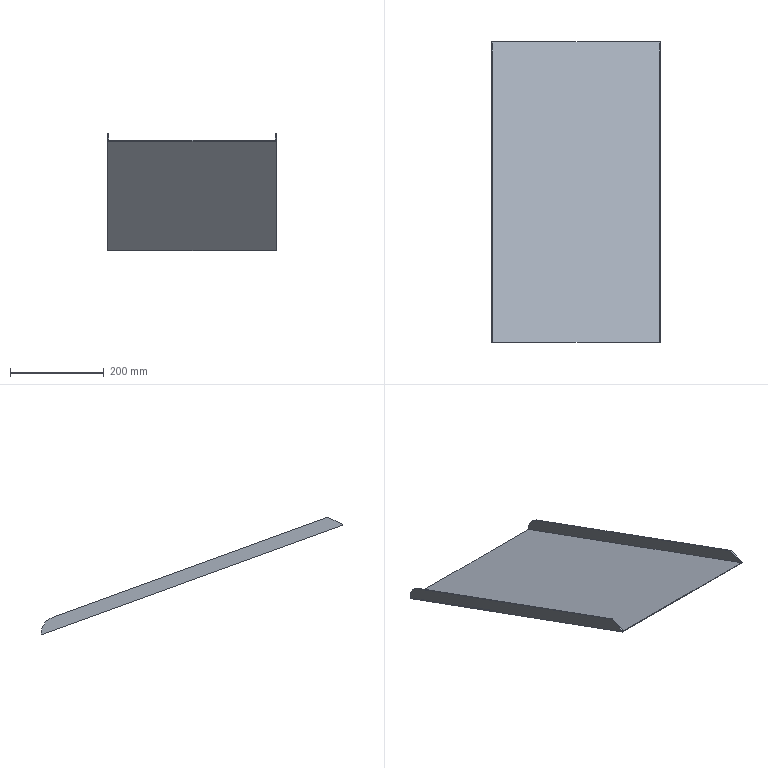Part | NX | features solid 2 | 1 solid | 14 faces | box 360 x 643.015 x 251.109 mm | volume 558969 mm3 | plane 12 | cylinder 2 | commonest cylinder face diameters 70 x2
STEP:
#1=CARTESIAN_POINT('',(-202.,620.,-449.011));
#2=VERTEX_POINT('',#1);
#3=CARTESIAN_POINT('',(-558.,620.,-449.011));
#4=VERTEX_POINT('',#3);
#5=CARTESIAN_POINT('',(-320.,620.,-449.011));
#6=DIRECTION('',(-1.,0.,0.));
#7=VECTOR('',#6,1000.);
#8=LINE('',#5,#7);
#9=EDGE_CURVE('',#2,#4,#8,.T.);
#10=ORIENTED_EDGE('',*,*,#9,.T.);
#11=CARTESIAN_POINT('',(-558.,-23.015,-214.973));
#12=VERTEX_POINT('',#11);
#13=CARTESIAN_POINT('',(-558.,-70.,-197.872));
#14=DIRECTION('',(0.,0.9397,-0.342));
#15=VECTOR('',#14,1000.);
#16=LINE('',#13,#15);
#17=EDGE_CURVE('',#12,#4,#16,.T.);
#18=ORIENTED_EDGE('',*,*,#17,.F.);
#19=CARTESIAN_POINT('',(-202.,-23.015,-214.973));
#20=VERTEX_POINT('',#19);
#21=CARTESIAN_POINT('',(-320.,-23.015,-214.973));
#22=DIRECTION('',(1.,0.,0.));
#23=VECTOR('',#22,1000.);
#24=LINE('',#21,#23);
#25=EDGE_CURVE('',#20,#12,#24,.F.);
#26=ORIENTED_EDGE('',*,*,#25,.F.);
#27=CARTESIAN_POINT('',(-202.,-70.,-197.872));
#28=DIRECTION('',(0.,0.9397,-0.342));
#29=VECTOR('',#28,1000.);
#30=LINE('',#27,#29);
#31=EDGE_CURVE('',#20,#2,#30,.T.);
#32=ORIENTED_EDGE('',*,*,#31,.T.);
#33=EDGE_LOOP('',(#10,#18,#26,#32));
#34=FACE_BOUND('',#33,.T.);
#35=CARTESIAN_POINT('',(-320.,-69.316,-198.121));
#36=DIRECTION('',(0.,-0.342,-0.9397));
#37=DIRECTION('',(-1.,0.,0.));
#38=AXIS2_PLACEMENT_3D('',#35,#36,#37);
#39=PLANE('',#38);
#40=ADVANCED_FACE('',(#34),#39,.F.);
#41=CARTESIAN_POINT('',(-202.,620.,-446.914));
#42=VERTEX_POINT('',#41);
#43=CARTESIAN_POINT('',(-202.,620.,-570.));
#44=DIRECTION('',(0.,0.,1.));
#45=VECTOR('',#44,1000.);
#46=LINE('',#43,#45);
#47=EDGE_CURVE('',#2,#42,#46,.T.);
#48=ORIENTED_EDGE('',*,*,#47,.T.);
#49=CARTESIAN_POINT('',(-200.,620.,-446.914));
#50=VERTEX_POINT('',#49);
#51=CARTESIAN_POINT('',(585.,620.,-446.914));
#52=DIRECTION('',(-1.,0.,0.));
#53=VECTOR('',#52,1000.);
#54=LINE('',#51,#53);
#55=EDGE_CURVE('',#42,#50,#54,.F.);
#56=ORIENTED_EDGE('',*,*,#55,.T.);
#57=CARTESIAN_POINT('',(-200.,620.,-451.139));
#58=VERTEX_POINT('',#57);
#59=CARTESIAN_POINT('',(-200.,620.,-570.));
#60=DIRECTION('',(0.,0.,-1.));
#61=VECTOR('',#60,1000.);
#62=LINE('',#59,#61);
#63=EDGE_CURVE('',#50,#58,#62,.T.);
#64=ORIENTED_EDGE('',*,*,#63,.T.);
#65=CARTESIAN_POINT('',(-560.,620.,-451.139));
#66=VERTEX_POINT('',#65);
#67=CARTESIAN_POINT('',(-320.,620.,-451.139));
#68=DIRECTION('',(-1.,0.,0.));
#69=VECTOR('',#68,1000.);
#70=LINE('',#67,#69);
#71=EDGE_CURVE('',#58,#66,#70,.T.);
#72=ORIENTED_EDGE('',*,*,#71,.T.);
#73=CARTESIAN_POINT('',(-560.,620.,-446.914));
#74=VERTEX_POINT('',#73);
#75=CARTESIAN_POINT('',(-560.,620.,-570.));
#76=DIRECTION('',(0.,0.,-1.));
#77=VECTOR('',#76,1000.);
#78=LINE('',#75,#77);
#79=EDGE_CURVE('',#74,#66,#78,.T.);
#80=ORIENTED_EDGE('',*,*,#79,.F.);
#81=CARTESIAN_POINT('',(-558.,620.,-446.914));
#82=VERTEX_POINT('',#81);
#83=CARTESIAN_POINT('',(585.,620.,-446.914));
#84=DIRECTION('',(-1.,0.,0.));
#85=VECTOR('',#84,1000.);
#86=LINE('',#83,#85);
#87=EDGE_CURVE('',#74,#82,#86,.F.);
#88=ORIENTED_EDGE('',*,*,#87,.T.);
#89=CARTESIAN_POINT('',(-558.,620.,-570.));
#90=DIRECTION('',(0.,0.,1.));
#91=VECTOR('',#90,1000.);
#92=LINE('',#89,#91);
#93=EDGE_CURVE('',#4,#82,#92,.T.);
#94=ORIENTED_EDGE('',*,*,#93,.F.);
#95=ORIENTED_EDGE('',*,*,#9,.F.);
#96=EDGE_LOOP('',(#48,#56,#64,#72,#80,#88,#94,#95));
#97=FACE_BOUND('',#96,.T.);
#98=CARTESIAN_POINT('',(585.,620.,-570.));
#99=DIRECTION('',(0.,-1.,0.));
#100=DIRECTION('',(-1.,0.,0.));
#101=AXIS2_PLACEMENT_3D('',#98,#99,#100);
#102=PLANE('',#101);
#103=ADVANCED_FACE('',(#97),#102,.F.);
#104=CARTESIAN_POINT('',(-200.,9.027,-200.031));
#105=VERTEX_POINT('',#104);
#106=CARTESIAN_POINT('',(-200.,596.971,-414.025));
#107=VERTEX_POINT('',#106);
#108=CARTESIAN_POINT('',(-200.,-61.449,-174.379));
#109=DIRECTION('',(0.,0.9397,-0.342));
#110=VECTOR('',#109,1000.);
#111=LINE('',#108,#110);
#112=EDGE_CURVE('',#105,#107,#111,.T.);
#113=ORIENTED_EDGE('',*,*,#112,.F.);
#114=CARTESIAN_POINT('',(-200.,-23.015,-214.973));
#115=VERTEX_POINT('',#114);
#116=CARTESIAN_POINT('',(-200.,-23.015,-214.973));
#117=DIRECTION('',(0.,0.9063,0.4226));
#118=VECTOR('',#117,1000.);
#119=LINE('',#116,#118);
#120=EDGE_CURVE('',#105,#115,#119,.F.);
#121=ORIENTED_EDGE('',*,*,#120,.T.);
#122=CARTESIAN_POINT('',(-200.,-23.015,-217.101));
#123=VERTEX_POINT('',#122);
#124=CARTESIAN_POINT('',(-200.,-23.015,-17.101));
#125=DIRECTION('',(0.,0.,1.));
#126=VECTOR('',#125,1000.);
#127=LINE('',#124,#126);
#128=EDGE_CURVE('',#115,#123,#127,.F.);
#129=ORIENTED_EDGE('',*,*,#128,.T.);
#130=CARTESIAN_POINT('',(-200.,-70.,-200.));
#131=DIRECTION('',(0.,0.9397,-0.342));
#132=VECTOR('',#131,1000.);
#133=LINE('',#130,#132);
#134=EDGE_CURVE('',#123,#58,#133,.T.);
#135=ORIENTED_EDGE('',*,*,#134,.T.);
#136=ORIENTED_EDGE('',*,*,#63,.F.);
#137=CARTESIAN_POINT('',(-200.,585.,-446.914));
#138=DIRECTION('',(-1.,0.,0.));
#139=DIRECTION('',(0.,0.,1.));
#140=AXIS2_PLACEMENT_3D('',#137,#138,#139);
#141=CIRCLE('',#140,35.);
#142=EDGE_CURVE('',#50,#107,#141,.F.);
#143=ORIENTED_EDGE('',*,*,#142,.T.);
#144=EDGE_LOOP('',(#113,#121,#129,#135,#136,#143));
#145=FACE_BOUND('',#144,.T.);
#146=CARTESIAN_POINT('',(-200.,-69.316,-198.121));
#147=DIRECTION('',(-1.,0.,0.));
#148=DIRECTION('',(0.,0.,1.));
#149=AXIS2_PLACEMENT_3D('',#146,#147,#148);
#150=PLANE('',#149);
#151=ADVANCED_FACE('',(#145),#150,.F.);
#152=CARTESIAN_POINT('',(-560.,-23.015,-217.101));
#153=VERTEX_POINT('',#152);
#154=CARTESIAN_POINT('',(-320.,-23.015,-217.101));
#155=DIRECTION('',(1.,0.,0.));
#156=VECTOR('',#155,1000.);
#157=LINE('',#154,#156);
#158=EDGE_CURVE('',#123,#153,#157,.F.);
#159=ORIENTED_EDGE('',*,*,#158,.F.);
#160=ORIENTED_EDGE('',*,*,#128,.F.);
#161=CARTESIAN_POINT('',(-320.,-23.015,-214.973));
#162=DIRECTION('',(1.,0.,0.));
#163=VECTOR('',#162,1000.);
#164=LINE('',#161,#163);
#165=EDGE_CURVE('',#115,#20,#164,.F.);
#166=ORIENTED_EDGE('',*,*,#165,.T.);
#167=ORIENTED_EDGE('',*,*,#25,.T.);
#168=CARTESIAN_POINT('',(-560.,-23.015,-214.973));
#169=VERTEX_POINT('',#168);
#170=CARTESIAN_POINT('',(-573.,-23.015,-214.973));
#171=DIRECTION('',(1.,0.,0.));
#172=VECTOR('',#171,1000.);
#173=LINE('',#170,#172);
#174=EDGE_CURVE('',#12,#169,#173,.F.);
#175=ORIENTED_EDGE('',*,*,#174,.T.);
#176=CARTESIAN_POINT('',(-560.,-23.015,-17.101));
#177=DIRECTION('',(0.,0.,1.));
#178=VECTOR('',#177,1000.);
#179=LINE('',#176,#178);
#180=EDGE_CURVE('',#169,#153,#179,.F.);
#181=ORIENTED_EDGE('',*,*,#180,.T.);
#182=EDGE_LOOP('',(#159,#160,#166,#167,#175,#181));
#183=FACE_BOUND('',#182,.T.);
#184=CARTESIAN_POINT('',(3075.,-23.015,-17.101));
#185=DIRECTION('',(0.,1.,0.));
#186=DIRECTION('',(0.,0.,1.));
#187=AXIS2_PLACEMENT_3D('',#184,#185,#186);
#188=PLANE('',#187);
#189=ADVANCED_FACE('',(#183),#188,.F.);
#190=ORIENTED_EDGE('',*,*,#180,.F.);
#191=CARTESIAN_POINT('',(-560.,9.027,-200.031));
#192=VERTEX_POINT('',#191);
#193=CARTESIAN_POINT('',(-560.,-22.549,-214.755));
#194=DIRECTION('',(0.,-0.9063,-0.4226));
#195=VECTOR('',#194,1000.);
#196=LINE('',#193,#195);
#197=EDGE_CURVE('',#169,#192,#196,.F.);
#198=ORIENTED_EDGE('',*,*,#197,.T.);
#199=CARTESIAN_POINT('',(-560.,596.971,-414.025));
#200=VERTEX_POINT('',#199);
#201=CARTESIAN_POINT('',(-560.,-61.449,-174.379));
#202=DIRECTION('',(0.,0.9397,-0.342));
#203=VECTOR('',#202,1000.);
#204=LINE('',#201,#203);
#205=EDGE_CURVE('',#192,#200,#204,.T.);
#206=ORIENTED_EDGE('',*,*,#205,.T.);
#207=CARTESIAN_POINT('',(-560.,585.,-446.914));
#208=DIRECTION('',(-1.,0.,0.));
#209=DIRECTION('',(0.,0.,1.));
#210=AXIS2_PLACEMENT_3D('',#207,#208,#209);
#211=CIRCLE('',#210,35.);
#212=EDGE_CURVE('',#200,#74,#211,.T.);
#213=ORIENTED_EDGE('',*,*,#212,.T.);
#214=ORIENTED_EDGE('',*,*,#79,.T.);
#215=CARTESIAN_POINT('',(-560.,-70.,-200.));
#216=DIRECTION('',(0.,0.9397,-0.342));
#217=VECTOR('',#216,1000.);
#218=LINE('',#215,#217);
#219=EDGE_CURVE('',#153,#66,#218,.T.);
#220=ORIENTED_EDGE('',*,*,#219,.F.);
#221=EDGE_LOOP('',(#190,#198,#206,#213,#214,#220));
#222=FACE_BOUND('',#221,.T.);
#223=CARTESIAN_POINT('',(-560.,-69.316,-198.121));
#224=DIRECTION('',(-1.,0.,0.));
#225=DIRECTION('',(0.,0.,1.));
#226=AXIS2_PLACEMENT_3D('',#223,#224,#225);
#227=PLANE('',#226);
#228=ADVANCED_FACE('',(#222),#227,.T.);
#229=ORIENTED_EDGE('',*,*,#71,.F.);
#230=ORIENTED_EDGE('',*,*,#134,.F.);
#231=ORIENTED_EDGE('',*,*,#158,.T.);
#232=ORIENTED_EDGE('',*,*,#219,.T.);
#233=EDGE_LOOP('',(#229,#230,#231,#232));
#234=FACE_BOUND('',#233,.T.);
#235=CARTESIAN_POINT('',(-320.,-70.,-200.));
#236=DIRECTION('',(0.,-0.342,-0.9397));
#237=DIRECTION('',(-1.,0.,0.));
#238=AXIS2_PLACEMENT_3D('',#235,#236,#237);
#239=PLANE('',#238);
#240=ADVANCED_FACE('',(#234),#239,.T.);
#241=CARTESIAN_POINT('',(-202.,9.027,-200.031));
#242=VERTEX_POINT('',#241);
#243=CARTESIAN_POINT('',(-202.,596.971,-414.025));
#244=VERTEX_POINT('',#243);
#245=CARTESIAN_POINT('',(-202.,-61.449,-174.379));
#246=DIRECTION('',(0.,0.9397,-0.342));
#247=VECTOR('',#246,1000.);
#248=LINE('',#245,#247);
#249=EDGE_CURVE('',#242,#244,#248,.T.);
#250=ORIENTED_EDGE('',*,*,#249,.F.);
#251=CARTESIAN_POINT('',(-320.,9.027,-200.031));
#252=DIRECTION('',(1.,0.,0.));
#253=VECTOR('',#252,1000.);
#254=LINE('',#251,#253);
#255=EDGE_CURVE('',#242,#105,#254,.T.);
#256=ORIENTED_EDGE('',*,*,#255,.T.);
#257=ORIENTED_EDGE('',*,*,#112,.T.);
#258=CARTESIAN_POINT('',(-320.,596.971,-414.025));
#259=DIRECTION('',(-1.,0.,0.));
#260=VECTOR('',#259,1000.);
#261=LINE('',#258,#260);
#262=EDGE_CURVE('',#107,#244,#261,.T.);
#263=ORIENTED_EDGE('',*,*,#262,.T.);
#264=EDGE_LOOP('',(#250,#256,#257,#263));
#265=FACE_BOUND('',#264,.T.);
#266=CARTESIAN_POINT('',(-320.,-61.449,-174.379));
#267=DIRECTION('',(0.,-0.342,-0.9397));
#268=DIRECTION('',(0.,0.9397,-0.342));
#269=AXIS2_PLACEMENT_3D('',#266,#267,#268);
#270=PLANE('',#269);
#271=ADVANCED_FACE('',(#265),#270,.F.);
#272=ORIENTED_EDGE('',*,*,#31,.F.);
#273=CARTESIAN_POINT('',(-202.,-23.015,-214.973));
#274=DIRECTION('',(0.,-0.9063,-0.4226));
#275=VECTOR('',#274,1000.);
#276=LINE('',#273,#275);
#277=EDGE_CURVE('',#20,#242,#276,.F.);
#278=ORIENTED_EDGE('',*,*,#277,.T.);
#279=ORIENTED_EDGE('',*,*,#249,.T.);
#280=CARTESIAN_POINT('',(-202.,585.,-446.914));
#281=DIRECTION('',(1.,0.,0.));
#282=DIRECTION('',(0.,0.,-1.));
#283=AXIS2_PLACEMENT_3D('',#280,#281,#282);
#284=CIRCLE('',#283,35.);
#285=EDGE_CURVE('',#244,#42,#284,.F.);
#286=ORIENTED_EDGE('',*,*,#285,.T.);
#287=ORIENTED_EDGE('',*,*,#47,.F.);
#288=EDGE_LOOP('',(#272,#278,#279,#286,#287));
#289=FACE_BOUND('',#288,.T.);
#290=CARTESIAN_POINT('',(-202.,-70.,-197.872));
#291=DIRECTION('',(1.,0.,0.));
#292=DIRECTION('',(0.,0.,-1.));
#293=AXIS2_PLACEMENT_3D('',#290,#291,#292);
#294=PLANE('',#293);
#295=ADVANCED_FACE('',(#289),#294,.F.);
#296=ORIENTED_EDGE('',*,*,#205,.F.);
#297=CARTESIAN_POINT('',(-558.,9.027,-200.031));
#298=VERTEX_POINT('',#297);
#299=CARTESIAN_POINT('',(-573.,9.027,-200.031));
#300=DIRECTION('',(1.,0.,0.));
#301=VECTOR('',#300,1000.);
#302=LINE('',#299,#301);
#303=EDGE_CURVE('',#192,#298,#302,.T.);
#304=ORIENTED_EDGE('',*,*,#303,.T.);
#305=CARTESIAN_POINT('',(-558.,596.971,-414.025));
#306=VERTEX_POINT('',#305);
#307=CARTESIAN_POINT('',(-558.,-61.449,-174.379));
#308=DIRECTION('',(0.,0.9397,-0.342));
#309=VECTOR('',#308,1000.);
#310=LINE('',#307,#309);
#311=EDGE_CURVE('',#298,#306,#310,.T.);
#312=ORIENTED_EDGE('',*,*,#311,.T.);
#313=CARTESIAN_POINT('',(-573.,596.971,-414.025));
#314=DIRECTION('',(-1.,0.,0.));
#315=VECTOR('',#314,1000.);
#316=LINE('',#313,#315);
#317=EDGE_CURVE('',#306,#200,#316,.T.);
#318=ORIENTED_EDGE('',*,*,#317,.T.);
#319=EDGE_LOOP('',(#296,#304,#312,#318));
#320=FACE_BOUND('',#319,.T.);
#321=CARTESIAN_POINT('',(-573.,-61.449,-174.379));
#322=DIRECTION('',(0.,-0.342,-0.9397));
#323=DIRECTION('',(0.,0.9397,-0.342));
#324=AXIS2_PLACEMENT_3D('',#321,#322,#323);
#325=PLANE('',#324);
#326=ADVANCED_FACE('',(#320),#325,.F.);
#327=ORIENTED_EDGE('',*,*,#311,.F.);
#328=CARTESIAN_POINT('',(-558.,-23.015,-214.973));
#329=DIRECTION('',(0.,0.9063,0.4226));
#330=VECTOR('',#329,1000.);
#331=LINE('',#328,#330);
#332=EDGE_CURVE('',#298,#12,#331,.F.);
#333=ORIENTED_EDGE('',*,*,#332,.T.);
#334=ORIENTED_EDGE('',*,*,#17,.T.);
#335=ORIENTED_EDGE('',*,*,#93,.T.);
#336=CARTESIAN_POINT('',(-558.,585.,-446.914));
#337=DIRECTION('',(1.,0.,0.));
#338=DIRECTION('',(0.,0.,-1.));
#339=AXIS2_PLACEMENT_3D('',#336,#337,#338);
#340=CIRCLE('',#339,35.);
#341=EDGE_CURVE('',#82,#306,#340,.T.);
#342=ORIENTED_EDGE('',*,*,#341,.T.);
#343=EDGE_LOOP('',(#327,#333,#334,#335,#342));
#344=FACE_BOUND('',#343,.T.);
#345=CARTESIAN_POINT('',(-558.,-70.,-197.872));
#346=DIRECTION('',(1.,0.,0.));
#347=DIRECTION('',(0.,0.,-1.));
#348=AXIS2_PLACEMENT_3D('',#345,#346,#347);
#349=PLANE('',#348);
#350=ADVANCED_FACE('',(#344),#349,.T.);
#351=ORIENTED_EDGE('',*,*,#341,.F.);
#352=ORIENTED_EDGE('',*,*,#87,.F.);
#353=ORIENTED_EDGE('',*,*,#212,.F.);
#354=ORIENTED_EDGE('',*,*,#317,.F.);
#355=EDGE_LOOP('',(#351,#352,#353,#354));
#356=FACE_BOUND('',#355,.T.);
#357=CARTESIAN_POINT('',(-573.,585.,-446.914));
#358=DIRECTION('',(-1.,0.,0.));
#359=DIRECTION('',(0.,0.,1.));
#360=AXIS2_PLACEMENT_3D('',#357,#358,#359);
#361=CYLINDRICAL_SURFACE('',#360,35.);
#362=ADVANCED_FACE('',(#356),#361,.T.);
#363=ORIENTED_EDGE('',*,*,#142,.F.);
#364=ORIENTED_EDGE('',*,*,#55,.F.);
#365=ORIENTED_EDGE('',*,*,#285,.F.);
#366=ORIENTED_EDGE('',*,*,#262,.F.);
#367=EDGE_LOOP('',(#363,#364,#365,#366));
#368=FACE_BOUND('',#367,.T.);
#369=CARTESIAN_POINT('',(-320.,585.,-446.914));
#370=DIRECTION('',(-1.,0.,0.));
#371=DIRECTION('',(0.,0.,1.));
#372=AXIS2_PLACEMENT_3D('',#369,#370,#371);
#373=CYLINDRICAL_SURFACE('',#372,35.);
#374=ADVANCED_FACE('',(#368),#373,.T.);
#375=ORIENTED_EDGE('',*,*,#332,.F.);
#376=ORIENTED_EDGE('',*,*,#303,.F.);
#377=ORIENTED_EDGE('',*,*,#197,.F.);
#378=ORIENTED_EDGE('',*,*,#174,.F.);
#379=EDGE_LOOP('',(#375,#376,#377,#378));
#380=FACE_BOUND('',#379,.T.);
#381=CARTESIAN_POINT('',(-573.,-23.015,-214.973));
#382=DIRECTION('',(0.,0.4226,-0.9063));
#383=DIRECTION('',(0.,0.9063,0.4226));
#384=AXIS2_PLACEMENT_3D('',#381,#382,#383);
#385=PLANE('',#384);
#386=ADVANCED_FACE('',(#380),#385,.F.);
#387=ORIENTED_EDGE('',*,*,#120,.F.);
#388=ORIENTED_EDGE('',*,*,#255,.F.);
#389=ORIENTED_EDGE('',*,*,#277,.F.);
#390=ORIENTED_EDGE('',*,*,#165,.F.);
#391=EDGE_LOOP('',(#387,#388,#389,#390));
#392=FACE_BOUND('',#391,.T.);
#393=CARTESIAN_POINT('',(-320.,-23.015,-214.973));
#394=DIRECTION('',(0.,0.4226,-0.9063));
#395=DIRECTION('',(0.,0.9063,0.4226));
#396=AXIS2_PLACEMENT_3D('',#393,#394,#395);
#397=PLANE('',#396);
#398=ADVANCED_FACE('',(#392),#397,.F.);
#399=CLOSED_SHELL('',(#40,#103,#151,#189,#228,#240,#271,#295,#326,#350,#362,#374,#386,#398));
#400=MANIFOLD_SOLID_BREP('',#399);
#401=(LENGTH_UNIT()NAMED_UNIT(*)SI_UNIT(.MILLI.,.METRE.));
#402=UNCERTAINTY_MEASURE_WITH_UNIT(LENGTH_MEASURE(0.00001),#401,'','');
#403=(NAMED_UNIT(*)PLANE_ANGLE_UNIT()SI_UNIT($,.RADIAN.));
#404=(NAMED_UNIT(*)SI_UNIT($,.STERADIAN.)SOLID_ANGLE_UNIT());
#405=(GEOMETRIC_REPRESENTATION_CONTEXT(3)GLOBAL_UNCERTAINTY_ASSIGNED_CONTEXT((#402))GLOBAL_UNIT_ASSIGNED_CONTEXT((#401,#403,#404))REPRESENTATION_CONTEXT('',''));
#406=ADVANCED_BREP_SHAPE_REPRESENTATION('',(#400),#405);